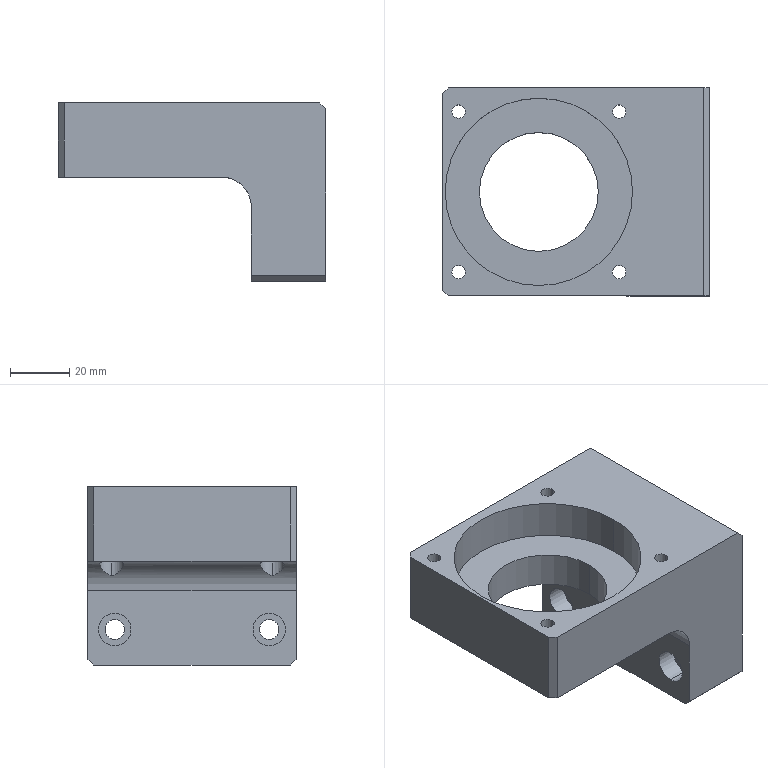Part | SolidWorks | features Cut 2, HoleWzd 2, Chamfer 1, Extrusion 1, Fillet 1 | 1 solid | 49 faces | box 90 x 70 x 60 mm | volume 158860 mm3 | cylinder 29 | plane 20 | commonest cylinder face diameters 4.5 x8 8 x8 6.6 x4 11 x4 40 x2 63 x2